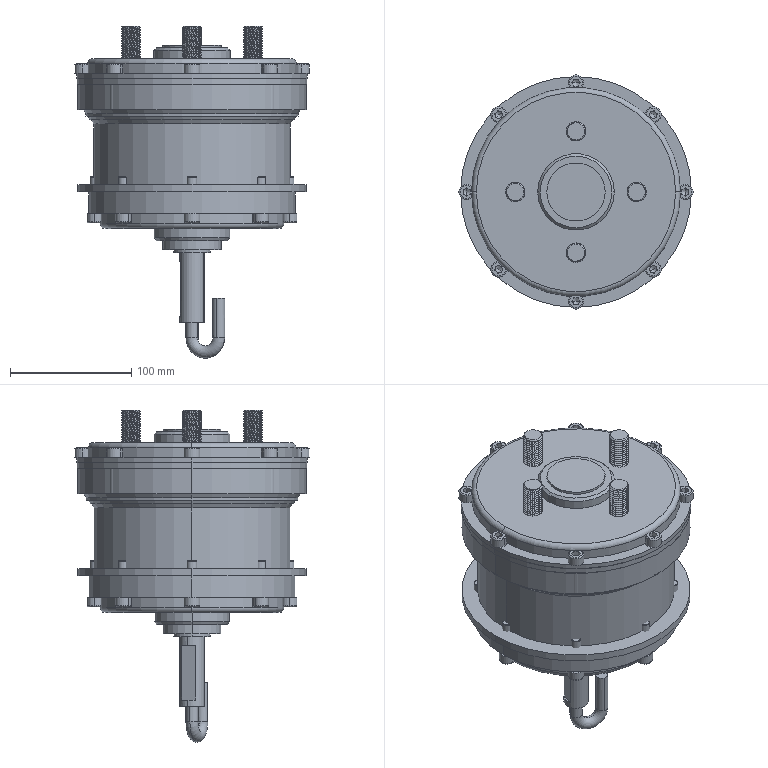Part | SolidWorks | features ReferencePattern 14, LocalCirPattern 1 | 22 solids | 680 faces | box 193 x 193 x 273.493 mm | volume 3354612 mm3 | plane 274 | cylinder 240 | cone 116 | torus 38 | spline 12 | commonest cylinder face diameters 16 x108 4.2 x32 8 x32 13 x32 10 x4 20 x4